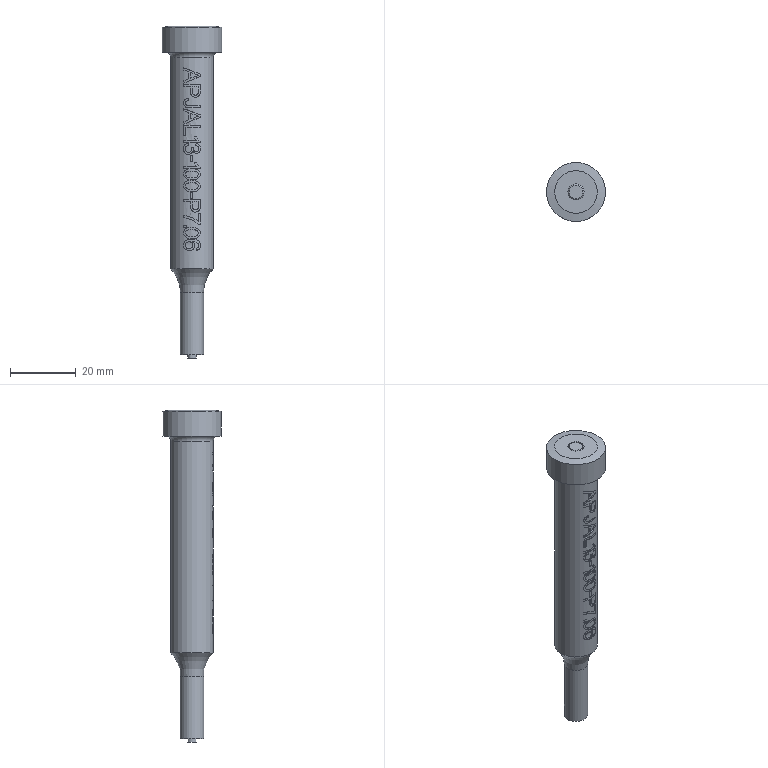Part | NX | features APJAL13-100-P7.06_2 2 | 1 solid | 211 faces | box 18 x 18 x 101 mm | volume 11860 mm3 | plane 120 | cylinder 86 | torus 2 | cone 2 | spline 1 | commonest cylinder face diameters 12.8 x17 13 x9 2.142 x3 2.555 x3 2.563 x3 2.593 x3